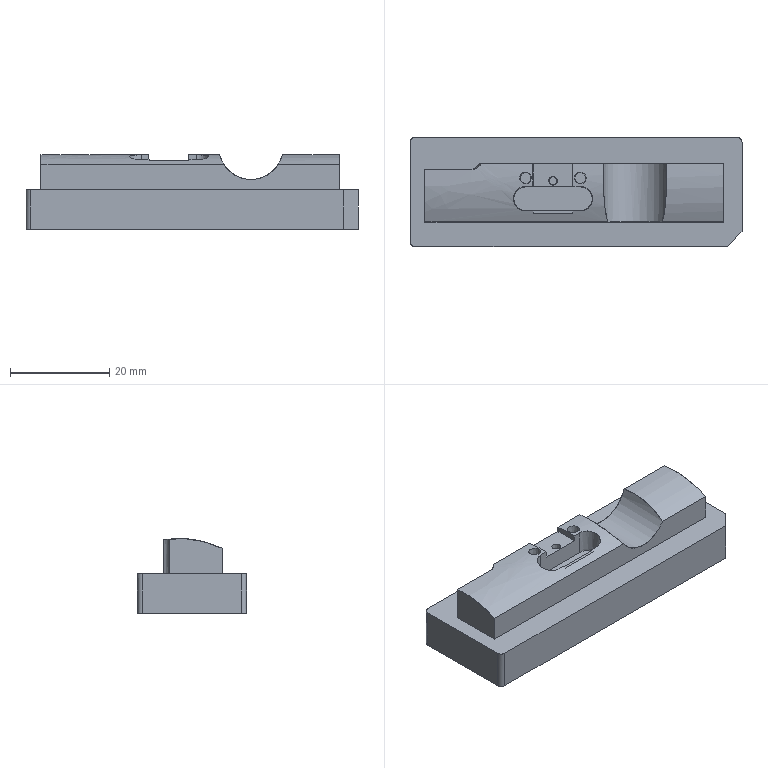CAM job | PowerMill | 3-axis milling, other | part box 67 x 22 x 15.086 mm
Tools:
number,name,type,diameter,tip_radius,length,cutting_length,overhang,flutes,holder,toolpaths_using
1,D10C,end_mill,10.0,0.0,60.0,,30.0,1,D42L35,2
15,D3C,end_mill,3.0,0.0,30.0,,15.0,1,D42L35,2
1,D10C_1_1,end_mill,10.0,0.0,60.0,,15.52,1,D42L35,6
15,D3C_1_1,end_mill,3.0,0.0,30.0,,7.28,1,D42L35,2
27,D1C_1_1,end_mill,1.0,0.0,5.12,,5.2,1,D42L35,1
3,D10_1_1,end_mill,10.0,0.0,60.0,,15.24,1,D42L35,6
22,R1.5_1_1,ball_nosed,3.0,1.5,30.0,,5.28,1,D42L35,2
10,D3_1_1_1_1,end_mill,3.0,0.0,30.0,,7.36,1,D42L35,4
8,D1_1_1,end_mill,1.0,0.0,5.28,,5.28,1,D42L35,4
13,Text_D4_1_1,taper_spherical,4.0,0.3,60.0,,7.36,1,D42L35,2
15,D3C_2_1,end_mill,3.0,0.0,30.0,,7.16,1,D42L35,2
27,D1C_2_1,end_mill,1.0,0.0,5.16,,5.24,1,D42L35,1
10,D3_1_1_1_2,end_mill,3.0,0.0,30.0,,7.2,1,D42L35,4
Operations:
program,toolpath,strategy,tool,tool_number,tool_diameter,tip_radius,flutes,spindle_rpm,feed_cut,surface_speed_m_min_computed,feed_per_tooth_computed,tolerance,thickness,stepover,stepdown,cut_length,cut_time_min,total_time_min,workplane
02-S-3-F,精公开粗01-扫面平行-D10C,raster_area_clear,D10C_1_1,1,10.0,0.0,1.0,8000.0,10000.0,251.33,1.25,0.03,0.28,6.0,1.0,462.92,0.046,0.0538,
02-S-3-F,精公开粗01-外形偏置-D10C,offset_area_clear,D10C_1_1,1,10.0,0.0,1.0,8000.0,10000.0,251.33,1.25,0.03,0.28,6.0,1.0,7536.937,0.754,0.8048,
02-S-3-F,精公开粗01-基准台等高-D10C,constantz,D10C_1_1,1,10.0,0.0,1.0,8000.0,10000.0,251.33,1.25,0.03,0.07,5.0,0.4,4549.041,0.455,0.4652,
02-S-3-F,精公再粗02-外形偏置-D3C,offset_area_clear,D3C_1_1,15,3.0,0.0,1.0,18000.0,5000.0,169.65,0.2778,0.03,0.0,2.0,1.0,9514.275,1.903,2.271,
02-S-3-F,精公再粗02-平行中光-D3C,raster,D3C_1_1,15,3.0,0.0,1.0,18000.0,5000.0,169.65,0.2778,0.03,0.0,0.15,1.0,5660.325,1.132,1.163,
02-S-3-F,精公再粗03-外形偏置-D1C,offset_area_clear,D1C_1_1,27,1.0,0.0,1.0,22000.0,2000.0,69.12,0.0909,0.03,0.0,0.5,1.0,1272.425,0.636,2.676,
02-S-3-F,精公基准台01-基准面偏置-D10,offset_area_clear,D10_1_1,3,10.0,0.0,1.0,8500.0,600.0,267.04,0.0706,0.005,0.38,5.0,1.0,186.841,0.311,0.3311,
02-S-3-F,精公基准台01-外形侧光-D10,profile_area_clear,D10_1_1,3,10.0,0.0,1.0,8500.0,600.0,267.04,0.0706,0.005,-0.07,0.08,1.0,348.648,0.581,0.6026,
02-S-3-F,精公基准台01-基准台侧光-D10,profile_area_clear,D10_1_1,3,10.0,0.0,1.0,8500.0,600.0,267.04,0.0706,0.005,0.0,0.08,1.0,413.234,0.689,0.7536,
02-S-3-F,精公精光01-平行-R1.5,raster,R1.5_1_1,22,3.0,1.5,1.0,22000.0,2000.0,207.35,0.0909,0.005,-0.075,0.04,1.0,16633.992,8.317,8.394,
02-S-3-F,精公精光02-平坦面平行-D3,raster_area_clear,D3_1_1_1_1,10,3.0,0.0,1.0,18000.0,600.0,169.65,0.0333,0.005,0.375,1.5,1.0,156.812,0.261,0.411,
02-S-3-F,精公精光02-等高-D3,constantz,D3_1_1_1_1,10,3.0,0.0,1.0,18000.0,2000.0,169.65,0.1111,0.005,-0.075,5.0,0.03,4737.714,2.369,2.458,
02-S-3-F,精公精光02-笔式-D3,pencil_corner,D3_1_1_1_1,10,3.0,0.0,1.0,18000.0,600.0,169.65,0.0333,0.005,-0.075,5.0,1.0,55.683,0.093,0.1254,
02-S-3-F,精公精光03-等高-D3_1,constantz,D3_1_1_1_1,10,3.0,0.0,1.0,18000.0,2000.0,169.65,0.1111,0.005,-0.075,5.0,0.03,856.373,0.428,0.6156,
02-S-3-F,精公精光04-等高-D1,constantz,D1_1_1,8,1.0,0.0,1.0,20000.0,1000.0,62.83,0.05,0.005,-0.075,5.0,0.02,2711.343,2.711,2.742,
02-S-3-F,精公精光04-平坦面偏置-D1,offset_area_clear,D1_1_1,8,1.0,0.0,1.0,20000.0,600.0,62.83,0.03,0.005,-0.03,0.5,1.0,12.868,0.021,0.0927,
02-S-3-F,精公刻字01-刻字-Text_D4,pattern,Text_D4_1_1,13,4.0,0.3,1.0,15000.0,1000.0,188.5,0.0667,0.005,0.0,5.0,1.0,49.984,0.05,0.0661,
02-S-3-R,粗公开粗01-扫面平行-D10C,raster_area_clear,D10C_1_1,1,10.0,0.0,1.0,8000.0,10000.0,251.33,1.25,0.03,0.15,6.0,1.0,922.2,0.092,0.1007,
02-S-3-R,粗公开粗01-外形偏置-D10C,offset_area_clear,D10C_1_1,1,10.0,0.0,1.0,8000.0,10000.0,251.33,1.25,0.03,0.15,6.0,1.0,7532.646,0.753,0.8045,
02-S-3-R,粗公开粗01-基准台等高-D10C,constantz,D10C_1_1,1,10.0,0.0,1.0,8000.0,10000.0,251.33,1.25,0.03,0.07,5.0,0.4,4549.041,0.455,0.4652,
02-S-3-R,粗公再粗02-外形偏置-D3C,offset_area_clear,D3C_2_1,15,3.0,0.0,1.0,18000.0,5000.0,169.65,0.2778,0.03,-0.13,2.0,1.0,8934.157,1.787,2.215,
02-S-3-R,粗公再粗02-平行中光-D3C,raster,D3C_2_1,15,3.0,0.0,1.0,18000.0,5000.0,169.65,0.2778,0.03,-0.13,0.15,1.0,5486.199,1.097,1.129,
02-S-3-R,粗公再粗03-外形偏置-D1C,offset_area_clear,D1C_2_1,27,1.0,0.0,1.0,22000.0,2000.0,69.12,0.0909,0.03,-0.13,0.5,1.0,1652.256,0.826,2.889,
02-S-3-R,粗公基准台01-基准面偏置-D10,offset_area_clear,D10_1_1,3,10.0,0.0,1.0,8500.0,600.0,267.04,0.0706,0.01,0.25,5.0,1.0,186.725,0.311,0.3308,
02-S-3-R,粗公基准台01-外形侧光-D10,profile_area_clear,D10_1_1,3,10.0,0.0,1.0,8500.0,600.0,267.04,0.0706,0.01,-0.2,0.08,1.0,347.018,0.578,0.5998,
02-S-3-R,粗公基准台01-基准台侧光-D10,profile_area_clear,D10_1_1,3,10.0,0.0,1.0,8500.0,600.0,267.04,0.0706,0.01,0.0,0.08,1.0,413.217,0.689,0.7536,
02-S-3-R,粗公精光01-平行-R1.5,raster,R1.5_1_1,22,3.0,1.5,1.0,22000.0,2000.0,207.35,0.0909,0.01,-0.205,0.048,1.0,13644.098,6.822,6.889,
02-S-3-R,粗公精光02-平坦面平行-D3,raster_area_clear,D3_1_1_1_2,10,3.0,0.0,1.0,18000.0,600.0,169.65,0.0333,0.01,0.245,1.5,1.0,157.107,0.262,0.4126,
02-S-3-R,粗公精光02-等高-D3,constantz,D3_1_1_1_2,10,3.0,0.0,1.0,18000.0,2000.0,169.65,0.1111,0.01,-0.205,5.0,0.036,4027.151,2.014,2.089,
02-S-3-R,粗公精光02-笔式-D3,pencil_corner,D3_1_1_1_2,10,3.0,0.0,1.0,18000.0,600.0,169.65,0.0333,0.01,-0.205,5.0,1.0,54.448,0.091,0.1257,
02-S-3-R,粗公精光03-等高-D3_1,constantz,D3_1_1_1_2,10,3.0,0.0,1.0,18000.0,2000.0,169.65,0.1111,0.01,-0.205,5.0,0.036,711.243,0.356,0.5137,
02-S-3-R,粗公精光04-等高-D1,constantz,D1_1_1,8,1.0,0.0,1.0,20000.0,1000.0,62.83,0.05,0.01,-0.205,5.0,0.024,2732.134,2.732,2.76,
02-S-3-R,粗公精光04-平坦面偏置-D1,offset_area_clear,D1_1_1,8,1.0,0.0,1.0,20000.0,600.0,62.83,0.03,0.01,-0.16,0.5,1.0,16.66,0.028,0.0991,
02-S-3-R,粗公刻字01-刻字-Text_D4,pattern,Text_D4_1_1,13,4.0,0.3,1.0,15000.0,1000.0,188.5,0.0667,0.01,0.0,5.0,1.0,45.471,0.045,0.0602,
,精公开粗01-外形偏置-D10C_Reference,offset_area_clear,D10C,1,10.0,0.0,1.0,8000.0,10000.0,251.33,1.25,0.03,0.28,6.0,1.0,19081.102,1.908,2.03,
,精公再粗02-外形偏置-D3C_Reference,offset_area_clear,D3C,15,3.0,0.0,1.0,18000.0,5000.0,169.65,0.2778,0.03,0.0,2.0,1.0,26918.001,5.384,6.53,
,粗公开粗01-外形偏置-D10C_Reference,offset_area_clear,D10C,1,10.0,0.0,1.0,8000.0,10000.0,251.33,1.25,0.03,0.15,6.0,1.0,18639.351,1.864,1.983,
,粗公再粗02-外形偏置-D3C_Reference,offset_area_clear,D3C,15,3.0,0.0,1.0,18000.0,5000.0,169.65,0.2778,0.03,-0.13,2.0,1.0,25929.476,5.186,6.429,